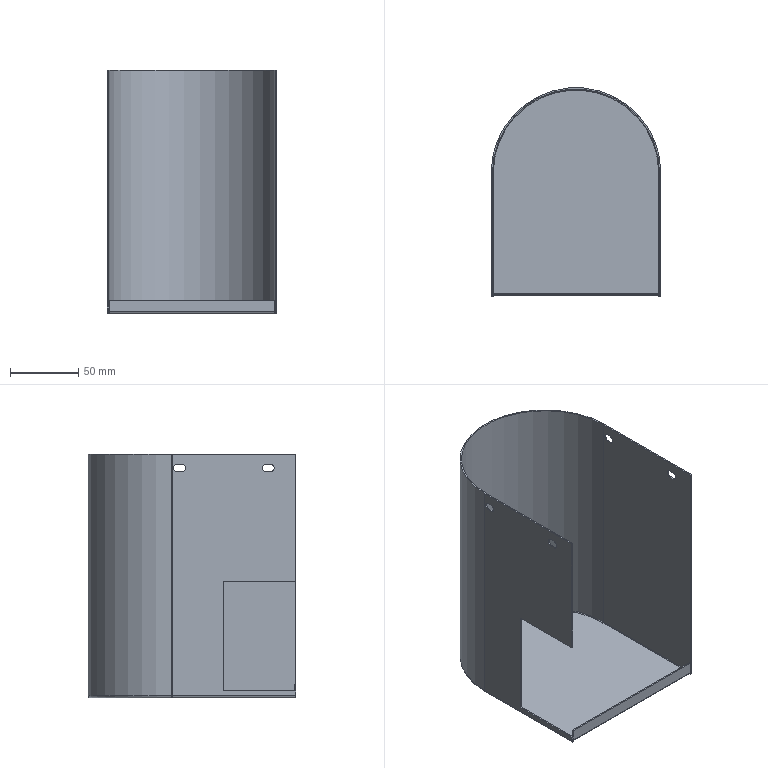Part | SolidWorks | features EdgeFlange 3, ICE 2, 3DProfileFeature 1, FlatPattern 1, SMBaseFlange 1, SheetMetal 1 | 1 solid | 66 faces | box 124 x 152 x 178 mm | volume 79554 mm3 | plane 46 | cylinder 16 | spline 2 | torus 2 | commonest cylinder face diameters 5.5 x8 1 x3 3 x3 122 x1 124 x1